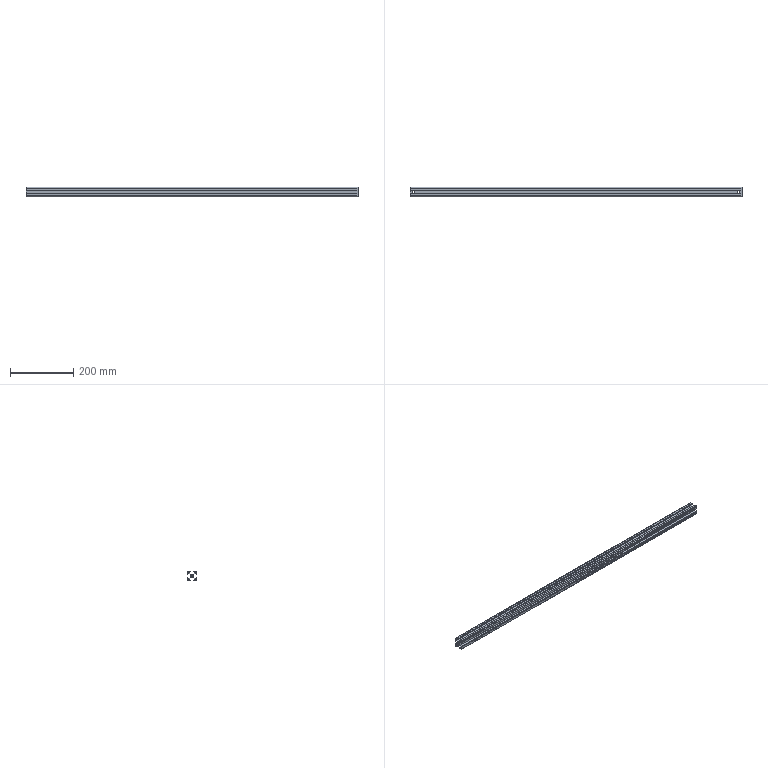Part | STEP file | 1 solid | 163 faces | box 1052 x 30 x 30 mm | volume 343124 mm3 | cylinder 85 | plane 78 | commonest cylinder face diameters 0.6 x55 2 x16 6.8 x6 5 x4 7 x4